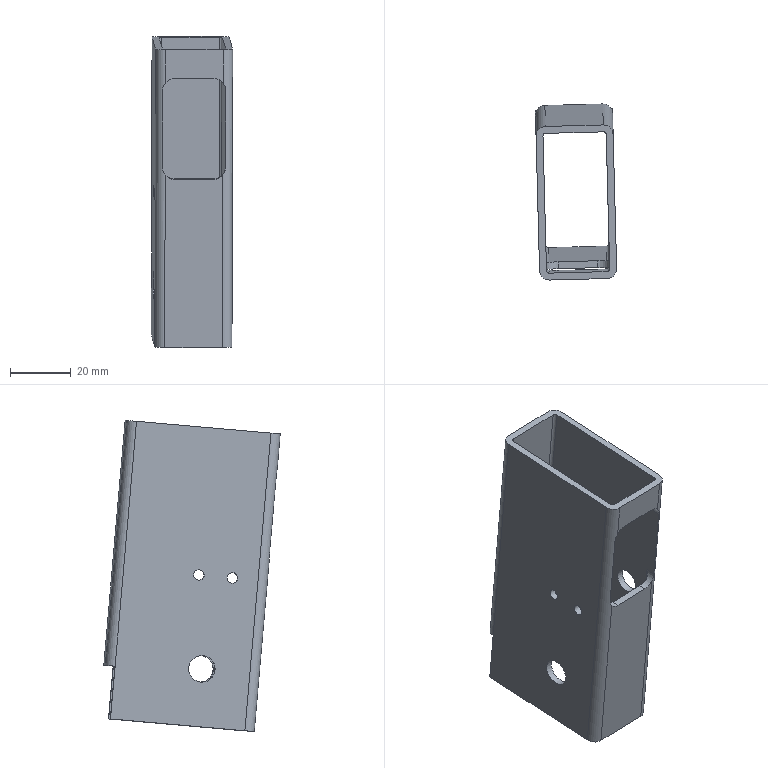Part | STEP file | 1_id786_x_t | 1 solid | 37 faces | box 26.767 x 58.14 x 102.478 mm | volume 28325 mm3 | cylinder 20 | plane 17 | commonest cylinder face diameters 1.778 x6 7.938 x6 6.35 x4 3.454 x2 8.731 x2